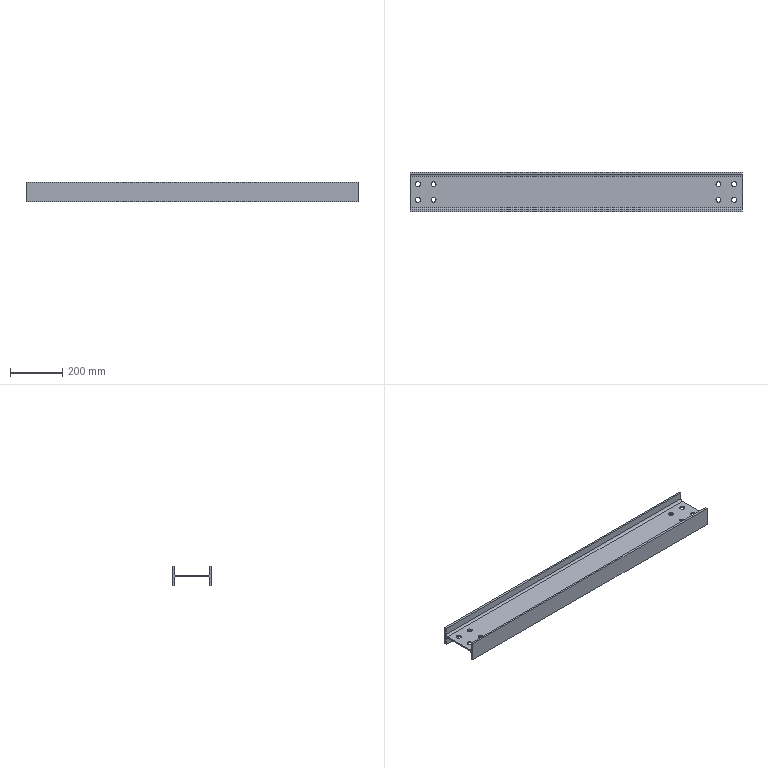Part | STEP file | 计量辅梁1主体_Default<As Machined> | 1 solid | 34 faces | box 1268 x 150 x 75 mm | volume 2251068 mm3 | cylinder 20 | plane 14 | commonest cylinder face diameters 19 x16 16 x4